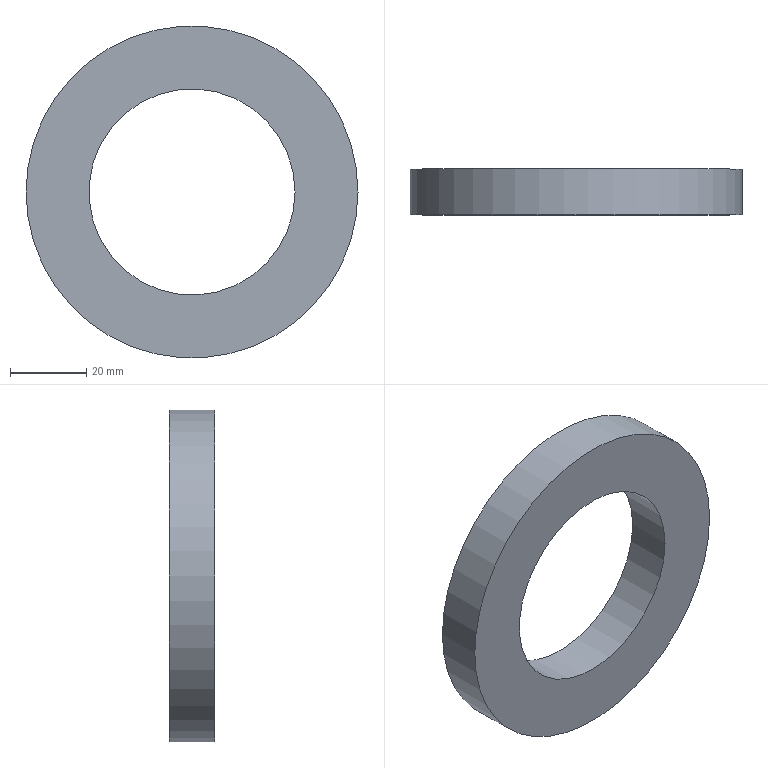Part | NX | features DATUM_CSYS 2, EXTRUDE 1, SKETCH 1 | 1 solid | 4 faces | box 87 x 12 x 87 mm | volume 43853 mm3 | cylinder 2 | plane 2 | commonest cylinder face diameters 54 x1 87 x1
STEP:
#1=CARTESIAN_POINT('',(43.5,-12.,0.));
#2=VERTEX_POINT('',#1);
#3=CARTESIAN_POINT('',(0.,-12.,0.));
#4=DIRECTION('',(0.,-1.,0.));
#5=DIRECTION('',(1.,0.,0.));
#6=AXIS2_PLACEMENT_3D('',#3,#4,#5);
#7=CIRCLE('',#6,43.5);
#8=EDGE_CURVE('',#2,#2,#7,.T.);
#9=ORIENTED_EDGE('',*,*,#8,.F.);
#10=EDGE_LOOP('',(#9));
#11=FACE_BOUND('',#10,.T.);
#12=CARTESIAN_POINT('',(43.5,0.,0.));
#13=VERTEX_POINT('',#12);
#14=CARTESIAN_POINT('',(0.,0.,0.));
#15=DIRECTION('',(0.,-1.,0.));
#16=DIRECTION('',(1.,0.,0.));
#17=AXIS2_PLACEMENT_3D('',#14,#15,#16);
#18=CIRCLE('',#17,43.5);
#19=EDGE_CURVE('',#13,#13,#18,.T.);
#20=ORIENTED_EDGE('',*,*,#19,.T.);
#21=EDGE_LOOP('',(#20));
#22=FACE_BOUND('',#21,.T.);
#23=CARTESIAN_POINT('',(0.,-12.,0.));
#24=DIRECTION('',(0.,1.,0.));
#25=DIRECTION('',(0.,0.,1.));
#26=AXIS2_PLACEMENT_3D('',#23,#24,#25);
#27=CYLINDRICAL_SURFACE('',#26,43.5);
#28=ADVANCED_FACE('',(#11,#22),#27,.T.);
#29=CARTESIAN_POINT('',(27.,-12.,0.));
#30=VERTEX_POINT('',#29);
#31=CARTESIAN_POINT('',(0.,-12.,0.));
#32=DIRECTION('',(0.,-1.,0.));
#33=DIRECTION('',(1.,0.,0.));
#34=AXIS2_PLACEMENT_3D('',#31,#32,#33);
#35=CIRCLE('',#34,27.);
#36=EDGE_CURVE('',#30,#30,#35,.T.);
#37=ORIENTED_EDGE('',*,*,#36,.T.);
#38=EDGE_LOOP('',(#37));
#39=FACE_BOUND('',#38,.T.);
#40=CARTESIAN_POINT('',(27.,0.,0.));
#41=VERTEX_POINT('',#40);
#42=CARTESIAN_POINT('',(0.,0.,0.));
#43=DIRECTION('',(0.,-1.,0.));
#44=DIRECTION('',(1.,0.,0.));
#45=AXIS2_PLACEMENT_3D('',#42,#43,#44);
#46=CIRCLE('',#45,27.);
#47=EDGE_CURVE('',#41,#41,#46,.T.);
#48=ORIENTED_EDGE('',*,*,#47,.F.);
#49=EDGE_LOOP('',(#48));
#50=FACE_BOUND('',#49,.T.);
#51=CARTESIAN_POINT('',(0.,-12.,0.));
#52=DIRECTION('',(0.,1.,0.));
#53=DIRECTION('',(0.,0.,1.));
#54=AXIS2_PLACEMENT_3D('',#51,#52,#53);
#55=CYLINDRICAL_SURFACE('',#54,27.);
#56=ADVANCED_FACE('',(#39,#50),#55,.F.);
#57=ORIENTED_EDGE('',*,*,#8,.T.);
#58=EDGE_LOOP('',(#57));
#59=FACE_BOUND('',#58,.T.);
#60=ORIENTED_EDGE('',*,*,#36,.F.);
#61=EDGE_LOOP('',(#60));
#62=FACE_BOUND('',#61,.T.);
#63=CARTESIAN_POINT('',(0.,-12.,0.));
#64=DIRECTION('',(0.,-1.,0.));
#65=DIRECTION('',(0.,0.,-1.));
#66=AXIS2_PLACEMENT_3D('',#63,#64,#65);
#67=PLANE('',#66);
#68=ADVANCED_FACE('',(#59,#62),#67,.T.);
#69=ORIENTED_EDGE('',*,*,#19,.F.);
#70=EDGE_LOOP('',(#69));
#71=FACE_BOUND('',#70,.T.);
#72=ORIENTED_EDGE('',*,*,#47,.T.);
#73=EDGE_LOOP('',(#72));
#74=FACE_BOUND('',#73,.T.);
#75=CARTESIAN_POINT('',(0.,0.,0.));
#76=DIRECTION('',(0.,-1.,0.));
#77=DIRECTION('',(0.,0.,-1.));
#78=AXIS2_PLACEMENT_3D('',#75,#76,#77);
#79=PLANE('',#78);
#80=ADVANCED_FACE('',(#71,#74),#79,.F.);
#81=CLOSED_SHELL('',(#28,#56,#68,#80));
#82=MANIFOLD_SOLID_BREP('',#81);
#83=(LENGTH_UNIT()NAMED_UNIT(*)SI_UNIT(.MILLI.,.METRE.));
#84=UNCERTAINTY_MEASURE_WITH_UNIT(LENGTH_MEASURE(0.00001),#83,'','');
#85=(NAMED_UNIT(*)PLANE_ANGLE_UNIT()SI_UNIT($,.RADIAN.));
#86=(NAMED_UNIT(*)SI_UNIT($,.STERADIAN.)SOLID_ANGLE_UNIT());
#87=(GEOMETRIC_REPRESENTATION_CONTEXT(3)GLOBAL_UNCERTAINTY_ASSIGNED_CONTEXT((#84))GLOBAL_UNIT_ASSIGNED_CONTEXT((#83,#85,#86))REPRESENTATION_CONTEXT('',''));
#88=ADVANCED_BREP_SHAPE_REPRESENTATION('',(#82),#87);